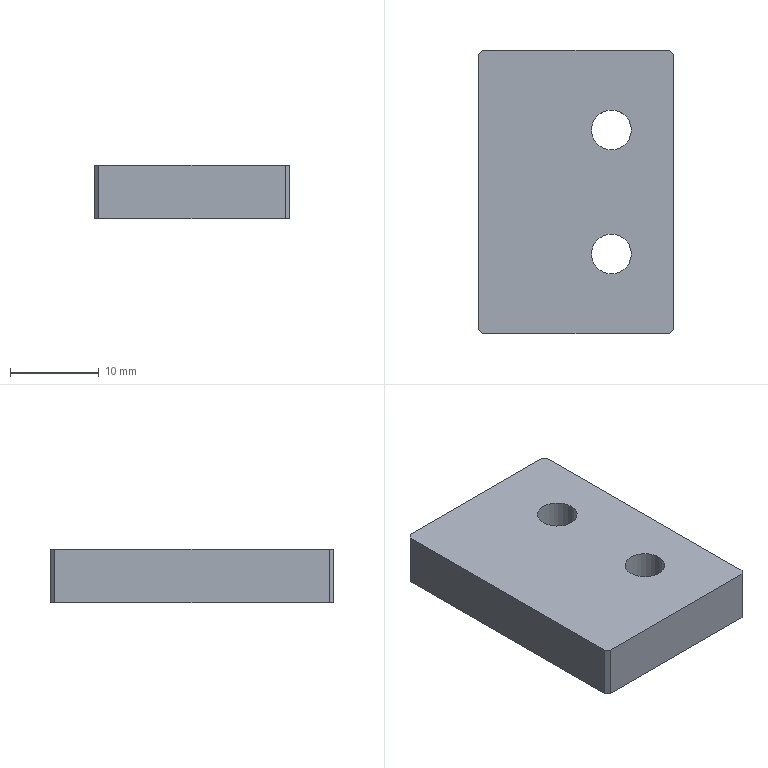Part | STEP file | PN_0014 Mount electronic clip cylinder pad block | 1 solid | 14 faces | box 22 x 32 x 6 mm | volume 4030 mm3 | plane 10 | cylinder 4 | commonest cylinder face diameters 4.5 x4
STEP:
#1=CARTESIAN_POINT('',(0.,0.,0.));
#2=DIRECTION('',(0.,0.,1.));
#3=DIRECTION('',(1.,0.,0.));
#4=AXIS2_PLACEMENT_3D('',#1,#2,#3);
#5=CARTESIAN_POINT('',(6.25,7.,0.));
#6=VERTEX_POINT('',#5);
#7=CARTESIAN_POINT('',(6.25,7.,6.));
#8=VERTEX_POINT('',#7);
#9=CARTESIAN_POINT('',(6.25,7.,6.));
#10=DIRECTION('',(0.,0.,1.));
#11=VECTOR('',#10,1.);
#12=LINE('',#9,#11);
#13=CARTESIAN_POINT('',(4.,7.,6.));
#14=DIRECTION('',(0.,0.,1.));
#15=DIRECTION('',(1.,0.,0.));
#16=AXIS2_PLACEMENT_3D('',#13,#14,#15);
#17=CYLINDRICAL_SURFACE('',#16,2.25);
#18=CARTESIAN_POINT('',(6.283,0.));
#19=DIRECTION('',(0.,1.));
#20=VECTOR('',#19,1.);
#21=LINE('',#18,#20);
#22=(GEOMETRIC_REPRESENTATION_CONTEXT(2)PARAMETRIC_REPRESENTATION_CONTEXT()REPRESENTATION_CONTEXT('',''));
#23=DEFINITIONAL_REPRESENTATION('',(#21),#22);
#24=PCURVE('',#17,#23);
#25=CARTESIAN_POINT('',(4.,7.,6.));
#26=DIRECTION('',(0.,0.,1.));
#27=DIRECTION('',(1.,0.,0.));
#28=AXIS2_PLACEMENT_3D('',#25,#26,#27);
#29=CYLINDRICAL_SURFACE('',#28,2.25);
#30=CARTESIAN_POINT('',(0.,0.));
#31=DIRECTION('',(0.,1.));
#32=VECTOR('',#31,1.);
#33=LINE('',#30,#32);
#34=(GEOMETRIC_REPRESENTATION_CONTEXT(2)PARAMETRIC_REPRESENTATION_CONTEXT()REPRESENTATION_CONTEXT('',''));
#35=DEFINITIONAL_REPRESENTATION('',(#33),#34);
#36=PCURVE('',#29,#35);
#37=SURFACE_CURVE('',#12,(#24,#36),.PCURVE_S1.);
#38=EDGE_CURVE('',#6,#8,#37,.T.);
#39=ORIENTED_EDGE('',*,*,#38,.T.);
#40=CARTESIAN_POINT('',(1.75,7.,6.));
#41=VERTEX_POINT('',#40);
#42=CARTESIAN_POINT('',(4.,7.,6.));
#43=DIRECTION('',(0.,0.,1.));
#44=DIRECTION('',(1.,0.,0.));
#45=AXIS2_PLACEMENT_3D('',#42,#43,#44);
#46=CIRCLE('',#45,2.25);
#47=CARTESIAN_POINT('',(0.,0.));
#48=DIRECTION('',(1.,0.));
#49=VECTOR('',#48,1.);
#50=LINE('',#47,#49);
#51=(GEOMETRIC_REPRESENTATION_CONTEXT(2)PARAMETRIC_REPRESENTATION_CONTEXT()REPRESENTATION_CONTEXT('',''));
#52=DEFINITIONAL_REPRESENTATION('',(#50),#51);
#53=PCURVE('',#17,#52);
#54=CARTESIAN_POINT('',(0.,0.,6.));
#55=DIRECTION('',(0.,0.,-1.));
#56=DIRECTION('',(-1.,0.,0.));
#57=AXIS2_PLACEMENT_3D('',#54,#55,#56);
#58=PLANE('',#57);
#59=CARTESIAN_POINT('',(-6.25,7.));
#60=CARTESIAN_POINT('',(-6.25,10.897));
#61=CARTESIAN_POINT('',(-2.875,8.949));
#62=CARTESIAN_POINT('',(0.5,7.));
#63=CARTESIAN_POINT('',(-2.875,5.051));
#64=CARTESIAN_POINT('',(-6.25,3.103));
#65=CARTESIAN_POINT('',(-6.25,7.));
#66=(BOUNDED_CURVE()B_SPLINE_CURVE(2,(#59,#60,#61,#62,#63,#64,#65),.UNSPECIFIED.,.T.,.F.)B_SPLINE_CURVE_WITH_KNOTS((1,2,2,2,2,1),(-2.094,0.,2.094,4.189,6.283,8.378),.UNSPECIFIED.)CURVE()GEOMETRIC_REPRESENTATION_ITEM()RATIONAL_B_SPLINE_CURVE((1.,0.5,1.,0.5,1.,0.5,1.))REPRESENTATION_ITEM(''));
#67=(GEOMETRIC_REPRESENTATION_CONTEXT(2)PARAMETRIC_REPRESENTATION_CONTEXT()REPRESENTATION_CONTEXT('',''));
#68=DEFINITIONAL_REPRESENTATION('',(#66),#67);
#69=PCURVE('',#58,#68);
#70=SURFACE_CURVE('',#46,(#53,#69),.PCURVE_S1.);
#71=EDGE_CURVE('',#41,#8,#70,.T.);
#72=ORIENTED_EDGE('',*,*,#71,.F.);
#73=CARTESIAN_POINT('',(1.75,7.,0.));
#74=VERTEX_POINT('',#73);
#75=CARTESIAN_POINT('',(1.75,7.,6.));
#76=DIRECTION('',(0.,0.,1.));
#77=VECTOR('',#76,1.);
#78=LINE('',#75,#77);
#79=CARTESIAN_POINT('',(3.142,0.));
#80=DIRECTION('',(0.,1.));
#81=VECTOR('',#80,1.);
#82=LINE('',#79,#81);
#83=(GEOMETRIC_REPRESENTATION_CONTEXT(2)PARAMETRIC_REPRESENTATION_CONTEXT()REPRESENTATION_CONTEXT('',''));
#84=DEFINITIONAL_REPRESENTATION('',(#82),#83);
#85=PCURVE('',#17,#84);
#86=CARTESIAN_POINT('',(3.142,0.));
#87=DIRECTION('',(0.,1.));
#88=VECTOR('',#87,1.);
#89=LINE('',#86,#88);
#90=(GEOMETRIC_REPRESENTATION_CONTEXT(2)PARAMETRIC_REPRESENTATION_CONTEXT()REPRESENTATION_CONTEXT('',''));
#91=DEFINITIONAL_REPRESENTATION('',(#89),#90);
#92=PCURVE('',#29,#91);
#93=SURFACE_CURVE('',#78,(#85,#92),.PCURVE_S1.);
#94=EDGE_CURVE('',#74,#41,#93,.T.);
#95=ORIENTED_EDGE('',*,*,#94,.F.);
#96=CARTESIAN_POINT('',(4.,7.,0.));
#97=DIRECTION('',(0.,0.,-1.));
#98=DIRECTION('',(-1.,0.,0.));
#99=AXIS2_PLACEMENT_3D('',#96,#97,#98);
#100=CIRCLE('',#99,2.25);
#101=CARTESIAN_POINT('',(9.425,-6.));
#102=DIRECTION('',(-1.,0.));
#103=VECTOR('',#102,1.);
#104=LINE('',#101,#103);
#105=(GEOMETRIC_REPRESENTATION_CONTEXT(2)PARAMETRIC_REPRESENTATION_CONTEXT()REPRESENTATION_CONTEXT('',''));
#106=DEFINITIONAL_REPRESENTATION('',(#104),#105);
#107=PCURVE('',#17,#106);
#108=CARTESIAN_POINT('',(0.,0.,0.));
#109=DIRECTION('',(0.,0.,-1.));
#110=DIRECTION('',(-1.,0.,0.));
#111=AXIS2_PLACEMENT_3D('',#108,#109,#110);
#112=PLANE('',#111);
#113=CARTESIAN_POINT('',(-4.,7.));
#114=DIRECTION('',(1.,0.));
#115=AXIS2_PLACEMENT_2D('',#113,#114);
#116=CIRCLE('',#115,2.25);
#117=(GEOMETRIC_REPRESENTATION_CONTEXT(2)PARAMETRIC_REPRESENTATION_CONTEXT()REPRESENTATION_CONTEXT('',''));
#118=DEFINITIONAL_REPRESENTATION('',(#116),#117);
#119=PCURVE('',#112,#118);
#120=SURFACE_CURVE('',#100,(#107,#119),.PCURVE_S1.);
#121=EDGE_CURVE('',#6,#74,#120,.T.);
#122=ORIENTED_EDGE('',*,*,#121,.F.);
#123=EDGE_LOOP('',(#39,#72,#95,#122));
#124=FACE_BOUND('',#123,.F.);
#125=ADVANCED_FACE('',(#124),#17,.F.);
#126=CARTESIAN_POINT('',(6.25,-7.,0.));
#127=VERTEX_POINT('',#126);
#128=CARTESIAN_POINT('',(6.25,-7.,6.));
#129=VERTEX_POINT('',#128);
#130=CARTESIAN_POINT('',(6.25,-7.,6.));
#131=DIRECTION('',(0.,0.,1.));
#132=VECTOR('',#131,1.);
#133=LINE('',#130,#132);
#134=CARTESIAN_POINT('',(4.,-7.,6.));
#135=DIRECTION('',(0.,0.,1.));
#136=DIRECTION('',(1.,0.,0.));
#137=AXIS2_PLACEMENT_3D('',#134,#135,#136);
#138=CYLINDRICAL_SURFACE('',#137,2.25);
#139=CARTESIAN_POINT('',(6.283,0.));
#140=DIRECTION('',(0.,1.));
#141=VECTOR('',#140,1.);
#142=LINE('',#139,#141);
#143=(GEOMETRIC_REPRESENTATION_CONTEXT(2)PARAMETRIC_REPRESENTATION_CONTEXT()REPRESENTATION_CONTEXT('',''));
#144=DEFINITIONAL_REPRESENTATION('',(#142),#143);
#145=PCURVE('',#138,#144);
#146=CARTESIAN_POINT('',(4.,-7.,6.));
#147=DIRECTION('',(0.,0.,1.));
#148=DIRECTION('',(1.,0.,0.));
#149=AXIS2_PLACEMENT_3D('',#146,#147,#148);
#150=CYLINDRICAL_SURFACE('',#149,2.25);
#151=CARTESIAN_POINT('',(0.,0.));
#152=DIRECTION('',(0.,1.));
#153=VECTOR('',#152,1.);
#154=LINE('',#151,#153);
#155=(GEOMETRIC_REPRESENTATION_CONTEXT(2)PARAMETRIC_REPRESENTATION_CONTEXT()REPRESENTATION_CONTEXT('',''));
#156=DEFINITIONAL_REPRESENTATION('',(#154),#155);
#157=PCURVE('',#150,#156);
#158=SURFACE_CURVE('',#133,(#145,#157),.PCURVE_S1.);
#159=EDGE_CURVE('',#127,#129,#158,.T.);
#160=ORIENTED_EDGE('',*,*,#159,.T.);
#161=CARTESIAN_POINT('',(1.75,-7.,6.));
#162=VERTEX_POINT('',#161);
#163=CARTESIAN_POINT('',(4.,-7.,6.));
#164=DIRECTION('',(0.,0.,1.));
#165=DIRECTION('',(1.,0.,0.));
#166=AXIS2_PLACEMENT_3D('',#163,#164,#165);
#167=CIRCLE('',#166,2.25);
#168=CARTESIAN_POINT('',(0.,0.));
#169=DIRECTION('',(1.,0.));
#170=VECTOR('',#169,1.);
#171=LINE('',#168,#170);
#172=(GEOMETRIC_REPRESENTATION_CONTEXT(2)PARAMETRIC_REPRESENTATION_CONTEXT()REPRESENTATION_CONTEXT('',''));
#173=DEFINITIONAL_REPRESENTATION('',(#171),#172);
#174=PCURVE('',#138,#173);
#175=CARTESIAN_POINT('',(-6.25,-7.));
#176=CARTESIAN_POINT('',(-6.25,-3.103));
#177=CARTESIAN_POINT('',(-2.875,-5.051));
#178=CARTESIAN_POINT('',(0.5,-7.));
#179=CARTESIAN_POINT('',(-2.875,-8.949));
#180=CARTESIAN_POINT('',(-6.25,-10.897));
#181=CARTESIAN_POINT('',(-6.25,-7.));
#182=(BOUNDED_CURVE()B_SPLINE_CURVE(2,(#175,#176,#177,#178,#179,#180,#181),.UNSPECIFIED.,.T.,.F.)B_SPLINE_CURVE_WITH_KNOTS((1,2,2,2,2,1),(-2.094,0.,2.094,4.189,6.283,8.378),.UNSPECIFIED.)CURVE()GEOMETRIC_REPRESENTATION_ITEM()RATIONAL_B_SPLINE_CURVE((1.,0.5,1.,0.5,1.,0.5,1.))REPRESENTATION_ITEM(''));
#183=(GEOMETRIC_REPRESENTATION_CONTEXT(2)PARAMETRIC_REPRESENTATION_CONTEXT()REPRESENTATION_CONTEXT('',''));
#184=DEFINITIONAL_REPRESENTATION('',(#182),#183);
#185=PCURVE('',#58,#184);
#186=SURFACE_CURVE('',#167,(#174,#185),.PCURVE_S1.);
#187=EDGE_CURVE('',#162,#129,#186,.T.);
#188=ORIENTED_EDGE('',*,*,#187,.F.);
#189=CARTESIAN_POINT('',(1.75,-7.,0.));
#190=VERTEX_POINT('',#189);
#191=CARTESIAN_POINT('',(1.75,-7.,6.));
#192=DIRECTION('',(0.,0.,1.));
#193=VECTOR('',#192,1.);
#194=LINE('',#191,#193);
#195=CARTESIAN_POINT('',(3.142,0.));
#196=DIRECTION('',(0.,1.));
#197=VECTOR('',#196,1.);
#198=LINE('',#195,#197);
#199=(GEOMETRIC_REPRESENTATION_CONTEXT(2)PARAMETRIC_REPRESENTATION_CONTEXT()REPRESENTATION_CONTEXT('',''));
#200=DEFINITIONAL_REPRESENTATION('',(#198),#199);
#201=PCURVE('',#138,#200);
#202=CARTESIAN_POINT('',(3.142,0.));
#203=DIRECTION('',(0.,1.));
#204=VECTOR('',#203,1.);
#205=LINE('',#202,#204);
#206=(GEOMETRIC_REPRESENTATION_CONTEXT(2)PARAMETRIC_REPRESENTATION_CONTEXT()REPRESENTATION_CONTEXT('',''));
#207=DEFINITIONAL_REPRESENTATION('',(#205),#206);
#208=PCURVE('',#150,#207);
#209=SURFACE_CURVE('',#194,(#201,#208),.PCURVE_S1.);
#210=EDGE_CURVE('',#190,#162,#209,.T.);
#211=ORIENTED_EDGE('',*,*,#210,.F.);
#212=CARTESIAN_POINT('',(4.,-7.,0.));
#213=DIRECTION('',(0.,0.,-1.));
#214=DIRECTION('',(-1.,0.,0.));
#215=AXIS2_PLACEMENT_3D('',#212,#213,#214);
#216=CIRCLE('',#215,2.25);
#217=CARTESIAN_POINT('',(9.425,-6.));
#218=DIRECTION('',(-1.,0.));
#219=VECTOR('',#218,1.);
#220=LINE('',#217,#219);
#221=(GEOMETRIC_REPRESENTATION_CONTEXT(2)PARAMETRIC_REPRESENTATION_CONTEXT()REPRESENTATION_CONTEXT('',''));
#222=DEFINITIONAL_REPRESENTATION('',(#220),#221);
#223=PCURVE('',#138,#222);
#224=CARTESIAN_POINT('',(-4.,-7.));
#225=DIRECTION('',(1.,0.));
#226=AXIS2_PLACEMENT_2D('',#224,#225);
#227=CIRCLE('',#226,2.25);
#228=(GEOMETRIC_REPRESENTATION_CONTEXT(2)PARAMETRIC_REPRESENTATION_CONTEXT()REPRESENTATION_CONTEXT('',''));
#229=DEFINITIONAL_REPRESENTATION('',(#227),#228);
#230=PCURVE('',#112,#229);
#231=SURFACE_CURVE('',#216,(#223,#230),.PCURVE_S1.);
#232=EDGE_CURVE('',#127,#190,#231,.T.);
#233=ORIENTED_EDGE('',*,*,#232,.F.);
#234=EDGE_LOOP('',(#160,#188,#211,#233));
#235=FACE_BOUND('',#234,.F.);
#236=ADVANCED_FACE('',(#235),#138,.F.);
#237=CARTESIAN_POINT('',(11.,-15.5,6.));
#238=VERTEX_POINT('',#237);
#239=CARTESIAN_POINT('',(11.,15.5,6.));
#240=VERTEX_POINT('',#239);
#241=CARTESIAN_POINT('',(11.,-16.,6.));
#242=DIRECTION('',(0.,1.,0.));
#243=VECTOR('',#242,1.);
#244=LINE('',#241,#243);
#245=CARTESIAN_POINT('',(11.,-16.,6.));
#246=DIRECTION('',(-1.,0.,0.));
#247=DIRECTION('',(0.,0.,1.));
#248=AXIS2_PLACEMENT_3D('',#245,#246,#247);
#249=PLANE('',#248);
#250=CARTESIAN_POINT('',(0.,0.));
#251=DIRECTION('',(0.,1.));
#252=VECTOR('',#251,1.);
#253=LINE('',#250,#252);
#254=(GEOMETRIC_REPRESENTATION_CONTEXT(2)PARAMETRIC_REPRESENTATION_CONTEXT()REPRESENTATION_CONTEXT('',''));
#255=DEFINITIONAL_REPRESENTATION('',(#253),#254);
#256=PCURVE('',#249,#255);
#257=CARTESIAN_POINT('',(-11.,-16.));
#258=DIRECTION('',(0.,1.));
#259=VECTOR('',#258,1.);
#260=LINE('',#257,#259);
#261=(GEOMETRIC_REPRESENTATION_CONTEXT(2)PARAMETRIC_REPRESENTATION_CONTEXT()REPRESENTATION_CONTEXT('',''));
#262=DEFINITIONAL_REPRESENTATION('',(#260),#261);
#263=PCURVE('',#58,#262);
#264=SURFACE_CURVE('',#244,(#256,#263),.PCURVE_S1.);
#265=EDGE_CURVE('',#238,#240,#264,.T.);
#266=ORIENTED_EDGE('',*,*,#265,.F.);
#267=CARTESIAN_POINT('',(11.,-15.5,0.));
#268=VERTEX_POINT('',#267);
#269=CARTESIAN_POINT('',(11.,-15.5,6.));
#270=DIRECTION('',(0.,0.,-1.));
#271=VECTOR('',#270,1.);
#272=LINE('',#269,#271);
#273=CARTESIAN_POINT('',(0.,0.5));
#274=DIRECTION('',(-1.,0.));
#275=VECTOR('',#274,1.);
#276=LINE('',#273,#275);
#277=(GEOMETRIC_REPRESENTATION_CONTEXT(2)PARAMETRIC_REPRESENTATION_CONTEXT()REPRESENTATION_CONTEXT('',''));
#278=DEFINITIONAL_REPRESENTATION('',(#276),#277);
#279=PCURVE('',#249,#278);
#280=CARTESIAN_POINT('',(11.,-15.5,6.));
#281=DIRECTION('',(-0.7071,0.7071,0.));
#282=DIRECTION('',(0.,0.,-1.));
#283=AXIS2_PLACEMENT_3D('',#280,#281,#282);
#284=PLANE('',#283);
#285=CARTESIAN_POINT('',(0.,0.));
#286=DIRECTION('',(1.,0.));
#287=VECTOR('',#286,1.);
#288=LINE('',#285,#287);
#289=(GEOMETRIC_REPRESENTATION_CONTEXT(2)PARAMETRIC_REPRESENTATION_CONTEXT()REPRESENTATION_CONTEXT('',''));
#290=DEFINITIONAL_REPRESENTATION('',(#288),#289);
#291=PCURVE('',#284,#290);
#292=SURFACE_CURVE('',#272,(#279,#291),.PCURVE_S1.);
#293=EDGE_CURVE('',#238,#268,#292,.T.);
#294=ORIENTED_EDGE('',*,*,#293,.T.);
#295=CARTESIAN_POINT('',(11.,15.5,0.));
#296=VERTEX_POINT('',#295);
#297=CARTESIAN_POINT('',(11.,-16.,0.));
#298=DIRECTION('',(0.,1.,0.));
#299=VECTOR('',#298,1.);
#300=LINE('',#297,#299);
#301=CARTESIAN_POINT('',(-6.,0.));
#302=DIRECTION('',(0.,1.));
#303=VECTOR('',#302,1.);
#304=LINE('',#301,#303);
#305=(GEOMETRIC_REPRESENTATION_CONTEXT(2)PARAMETRIC_REPRESENTATION_CONTEXT()REPRESENTATION_CONTEXT('',''));
#306=DEFINITIONAL_REPRESENTATION('',(#304),#305);
#307=PCURVE('',#249,#306);
#308=CARTESIAN_POINT('',(-11.,-16.));
#309=DIRECTION('',(0.,1.));
#310=VECTOR('',#309,1.);
#311=LINE('',#308,#310);
#312=(GEOMETRIC_REPRESENTATION_CONTEXT(2)PARAMETRIC_REPRESENTATION_CONTEXT()REPRESENTATION_CONTEXT('',''));
#313=DEFINITIONAL_REPRESENTATION('',(#311),#312);
#314=PCURVE('',#112,#313);
#315=SURFACE_CURVE('',#300,(#307,#314),.PCURVE_S1.);
#316=EDGE_CURVE('',#268,#296,#315,.T.);
#317=ORIENTED_EDGE('',*,*,#316,.T.);
#318=CARTESIAN_POINT('',(11.,15.5,6.));
#319=DIRECTION('',(0.,0.,1.));
#320=VECTOR('',#319,1.);
#321=LINE('',#318,#320);
#322=CARTESIAN_POINT('',(0.,31.5));
#323=DIRECTION('',(1.,0.));
#324=VECTOR('',#323,1.);
#325=LINE('',#322,#324);
#326=(GEOMETRIC_REPRESENTATION_CONTEXT(2)PARAMETRIC_REPRESENTATION_CONTEXT()REPRESENTATION_CONTEXT('',''));
#327=DEFINITIONAL_REPRESENTATION('',(#325),#326);
#328=PCURVE('',#249,#327);
#329=CARTESIAN_POINT('',(10.5,16.,6.));
#330=DIRECTION('',(-0.7071,-0.7071,0.));
#331=DIRECTION('',(0.,0.,-1.));
#332=AXIS2_PLACEMENT_3D('',#329,#330,#331);
#333=PLANE('',#332);
#334=CARTESIAN_POINT('',(0.,0.7071));
#335=DIRECTION('',(-1.,0.));
#336=VECTOR('',#335,1.);
#337=LINE('',#334,#336);
#338=(GEOMETRIC_REPRESENTATION_CONTEXT(2)PARAMETRIC_REPRESENTATION_CONTEXT()REPRESENTATION_CONTEXT('',''));
#339=DEFINITIONAL_REPRESENTATION('',(#337),#338);
#340=PCURVE('',#333,#339);
#341=SURFACE_CURVE('',#321,(#328,#340),.PCURVE_S1.);
#342=EDGE_CURVE('',#296,#240,#341,.T.);
#343=ORIENTED_EDGE('',*,*,#342,.T.);
#344=EDGE_LOOP('',(#266,#294,#317,#343));
#345=FACE_BOUND('',#344,.T.);
#346=ADVANCED_FACE('',(#345),#249,.F.);
#347=CARTESIAN_POINT('',(10.5,16.,0.));
#348=VERTEX_POINT('',#347);
#349=CARTESIAN_POINT('',(-10.5,16.,0.));
#350=VERTEX_POINT('',#349);
#351=CARTESIAN_POINT('',(-11.,16.,0.));
#352=DIRECTION('',(-1.,0.,0.));
#353=VECTOR('',#352,1.);
#354=LINE('',#351,#353);
#355=CARTESIAN_POINT('',(-11.,16.,6.));
#356=DIRECTION('',(0.,-1.,0.));
#357=DIRECTION('',(0.,0.,-1.));
#358=AXIS2_PLACEMENT_3D('',#355,#356,#357);
#359=PLANE('',#358);
#360=CARTESIAN_POINT('',(6.,0.));
#361=DIRECTION('',(0.,-1.));
#362=VECTOR('',#361,1.);
#363=LINE('',#360,#362);
#364=(GEOMETRIC_REPRESENTATION_CONTEXT(2)PARAMETRIC_REPRESENTATION_CONTEXT()REPRESENTATION_CONTEXT('',''));
#365=DEFINITIONAL_REPRESENTATION('',(#363),#364);
#366=PCURVE('',#359,#365);
#367=CARTESIAN_POINT('',(11.,16.));
#368=DIRECTION('',(1.,0.));
#369=VECTOR('',#368,1.);
#370=LINE('',#367,#369);
#371=(GEOMETRIC_REPRESENTATION_CONTEXT(2)PARAMETRIC_REPRESENTATION_CONTEXT()REPRESENTATION_CONTEXT('',''));
#372=DEFINITIONAL_REPRESENTATION('',(#370),#371);
#373=PCURVE('',#112,#372);
#374=SURFACE_CURVE('',#354,(#366,#373),.PCURVE_S1.);
#375=EDGE_CURVE('',#348,#350,#374,.T.);
#376=ORIENTED_EDGE('',*,*,#375,.T.);
#377=CARTESIAN_POINT('',(-10.5,16.,6.));
#378=VERTEX_POINT('',#377);
#379=CARTESIAN_POINT('',(-10.5,16.,6.));
#380=DIRECTION('',(0.,0.,1.));
#381=VECTOR('',#380,1.);
#382=LINE('',#379,#381);
#383=CARTESIAN_POINT('',(0.,0.5));
#384=DIRECTION('',(-1.,0.));
#385=VECTOR('',#384,1.);
#386=LINE('',#383,#385);
#387=(GEOMETRIC_REPRESENTATION_CONTEXT(2)PARAMETRIC_REPRESENTATION_CONTEXT()REPRESENTATION_CONTEXT('',''));
#388=DEFINITIONAL_REPRESENTATION('',(#386),#387);
#389=PCURVE('',#359,#388);
#390=CARTESIAN_POINT('',(-11.,15.5,6.));
#391=DIRECTION('',(0.7071,-0.7071,0.));
#392=DIRECTION('',(0.,0.,-1.));
#393=AXIS2_PLACEMENT_3D('',#390,#391,#392);
#394=PLANE('',#393);
#395=CARTESIAN_POINT('',(0.,0.7071));
#396=DIRECTION('',(-1.,0.));
#397=VECTOR('',#396,1.);
#398=LINE('',#395,#397);
#399=(GEOMETRIC_REPRESENTATION_CONTEXT(2)PARAMETRIC_REPRESENTATION_CONTEXT()REPRESENTATION_CONTEXT('',''));
#400=DEFINITIONAL_REPRESENTATION('',(#398),#399);
#401=PCURVE('',#394,#400);
#402=SURFACE_CURVE('',#382,(#389,#401),.PCURVE_S1.);
#403=EDGE_CURVE('',#350,#378,#402,.T.);
#404=ORIENTED_EDGE('',*,*,#403,.T.);
#405=CARTESIAN_POINT('',(10.5,16.,6.));
#406=VERTEX_POINT('',#405);
#407=CARTESIAN_POINT('',(-11.,16.,6.));
#408=DIRECTION('',(-1.,0.,0.));
#409=VECTOR('',#408,1.);
#410=LINE('',#407,#409);
#411=CARTESIAN_POINT('',(0.,0.));
#412=DIRECTION('',(0.,-1.));
#413=VECTOR('',#412,1.);
#414=LINE('',#411,#413);
#415=(GEOMETRIC_REPRESENTATION_CONTEXT(2)PARAMETRIC_REPRESENTATION_CONTEXT()REPRESENTATION_CONTEXT('',''));
#416=DEFINITIONAL_REPRESENTATION('',(#414),#415);
#417=PCURVE('',#359,#416);
#418=CARTESIAN_POINT('',(11.,16.));
#419=DIRECTION('',(1.,0.));
#420=VECTOR('',#419,1.);
#421=LINE('',#418,#420);
#422=(GEOMETRIC_REPRESENTATION_CONTEXT(2)PARAMETRIC_REPRESENTATION_CONTEXT()REPRESENTATION_CONTEXT('',''));
#423=DEFINITIONAL_REPRESENTATION('',(#421),#422);
#424=PCURVE('',#58,#423);
#425=SURFACE_CURVE('',#410,(#417,#424),.PCURVE_S1.);
#426=EDGE_CURVE('',#406,#378,#425,.T.);
#427=ORIENTED_EDGE('',*,*,#426,.F.);
#428=CARTESIAN_POINT('',(10.5,16.,6.));
#429=DIRECTION('',(0.,0.,-1.));
#430=VECTOR('',#429,1.);
#431=LINE('',#428,#430);
#432=CARTESIAN_POINT('',(0.,21.5));
#433=DIRECTION('',(1.,0.));
#434=VECTOR('',#433,1.);
#435=LINE('',#432,#434);
#436=(GEOMETRIC_REPRESENTATION_CONTEXT(2)PARAMETRIC_REPRESENTATION_CONTEXT()REPRESENTATION_CONTEXT('',''));
#437=DEFINITIONAL_REPRESENTATION('',(#435),#436);
#438=PCURVE('',#359,#437);
#439=CARTESIAN_POINT('',(0.,0.));
#440=DIRECTION('',(1.,0.));
#441=VECTOR('',#440,1.);
#442=LINE('',#439,#441);
#443=(GEOMETRIC_REPRESENTATION_CONTEXT(2)PARAMETRIC_REPRESENTATION_CONTEXT()REPRESENTATION_CONTEXT('',''));
#444=DEFINITIONAL_REPRESENTATION('',(#442),#443);
#445=PCURVE('',#333,#444);
#446=SURFACE_CURVE('',#431,(#438,#445),.PCURVE_S1.);
#447=EDGE_CURVE('',#406,#348,#446,.T.);
#448=ORIENTED_EDGE('',*,*,#447,.T.);
#449=EDGE_LOOP('',(#376,#404,#427,#448));
#450=FACE_BOUND('',#449,.T.);
#451=ADVANCED_FACE('',(#450),#359,.F.);
#452=CARTESIAN_POINT('',(-11.,15.5,0.));
#453=VERTEX_POINT('',#452);
#454=CARTESIAN_POINT('',(-11.,-15.5,0.));
#455=VERTEX_POINT('',#454);
#456=CARTESIAN_POINT('',(-11.,-16.,0.));
#457=DIRECTION('',(0.,-1.,0.));
#458=VECTOR('',#457,1.);
#459=LINE('',#456,#458);
#460=CARTESIAN_POINT('',(-11.,-16.,6.));
#461=DIRECTION('',(1.,0.,0.));
#462=DIRECTION('',(0.,0.,-1.));
#463=AXIS2_PLACEMENT_3D('',#460,#461,#462);
#464=PLANE('',#463);
#465=CARTESIAN_POINT('',(6.,0.));
#466=DIRECTION('',(0.,-1.));
#467=VECTOR('',#466,1.);
#468=LINE('',#465,#467);
#469=(GEOMETRIC_REPRESENTATION_CONTEXT(2)PARAMETRIC_REPRESENTATION_CONTEXT()REPRESENTATION_CONTEXT('',''));
#470=DEFINITIONAL_REPRESENTATION('',(#468),#469);
#471=PCURVE('',#464,#470);
#472=CARTESIAN_POINT('',(11.,-16.));
#473=DIRECTION('',(0.,-1.));
#474=VECTOR('',#473,1.);
#475=LINE('',#472,#474);
#476=(GEOMETRIC_REPRESENTATION_CONTEXT(2)PARAMETRIC_REPRESENTATION_CONTEXT()REPRESENTATION_CONTEXT('',''));
#477=DEFINITIONAL_REPRESENTATION('',(#475),#476);
#478=PCURVE('',#112,#477);
#479=SURFACE_CURVE('',#459,(#471,#478),.PCURVE_S1.);
#480=EDGE_CURVE('',#453,#455,#479,.T.);
#481=ORIENTED_EDGE('',*,*,#480,.T.);
#482=CARTESIAN_POINT('',(-11.,-15.5,6.));
#483=VERTEX_POINT('',#482);
#484=CARTESIAN_POINT('',(-11.,-15.5,6.));
#485=DIRECTION('',(0.,0.,1.));
#486=VECTOR('',#485,1.);
#487=LINE('',#484,#486);
#488=CARTESIAN_POINT('',(0.,0.5));
#489=DIRECTION('',(-1.,0.));
#490=VECTOR('',#489,1.);
#491=LINE('',#488,#490);
#492=(GEOMETRIC_REPRESENTATION_CONTEXT(2)PARAMETRIC_REPRESENTATION_CONTEXT()REPRESENTATION_CONTEXT('',''));
#493=DEFINITIONAL_REPRESENTATION('',(#491),#492);
#494=PCURVE('',#464,#493);
#495=CARTESIAN_POINT('',(-10.5,-16.,6.));
#496=DIRECTION('',(0.7071,0.7071,0.));
#497=DIRECTION('',(0.,0.,-1.));
#498=AXIS2_PLACEMENT_3D('',#495,#496,#497);
#499=PLANE('',#498);
#500=CARTESIAN_POINT('',(0.,0.7071));
#501=DIRECTION('',(-1.,0.));
#502=VECTOR('',#501,1.);
#503=LINE('',#500,#502);
#504=(GEOMETRIC_REPRESENTATION_CONTEXT(2)PARAMETRIC_REPRESENTATION_CONTEXT()REPRESENTATION_CONTEXT('',''));
#505=DEFINITIONAL_REPRESENTATION('',(#503),#504);
#506=PCURVE('',#499,#505);
#507=SURFACE_CURVE('',#487,(#494,#506),.PCURVE_S1.);
#508=EDGE_CURVE('',#455,#483,#507,.T.);
#509=ORIENTED_EDGE('',*,*,#508,.T.);
#510=CARTESIAN_POINT('',(-11.,15.5,6.));
#511=VERTEX_POINT('',#510);
#512=CARTESIAN_POINT('',(-11.,-16.,6.));
#513=DIRECTION('',(0.,-1.,0.));
#514=VECTOR('',#513,1.);
#515=LINE('',#512,#514);
#516=CARTESIAN_POINT('',(0.,0.));
#517=DIRECTION('',(0.,-1.));
#518=VECTOR('',#517,1.);
#519=LINE('',#516,#518);
#520=(GEOMETRIC_REPRESENTATION_CONTEXT(2)PARAMETRIC_REPRESENTATION_CONTEXT()REPRESENTATION_CONTEXT('',''));
#521=DEFINITIONAL_REPRESENTATION('',(#519),#520);
#522=PCURVE('',#464,#521);
#523=CARTESIAN_POINT('',(11.,-16.));
#524=DIRECTION('',(0.,-1.));
#525=VECTOR('',#524,1.);
#526=LINE('',#523,#525);
#527=(GEOMETRIC_REPRESENTATION_CONTEXT(2)PARAMETRIC_REPRESENTATION_CONTEXT()REPRESENTATION_CONTEXT('',''));
#528=DEFINITIONAL_REPRESENTATION('',(#526),#527);
#529=PCURVE('',#58,#528);
#530=SURFACE_CURVE('',#515,(#522,#529),.PCURVE_S1.);
#531=EDGE_CURVE('',#511,#483,#530,.T.);
#532=ORIENTED_EDGE('',*,*,#531,.F.);
#533=CARTESIAN_POINT('',(-11.,15.5,6.));
#534=DIRECTION('',(0.,0.,-1.));
#535=VECTOR('',#534,1.);
#536=LINE('',#533,#535);
#537=CARTESIAN_POINT('',(0.,31.5));
#538=DIRECTION('',(1.,0.));
#539=VECTOR('',#538,1.);
#540=LINE('',#537,#539);
#541=(GEOMETRIC_REPRESENTATION_CONTEXT(2)PARAMETRIC_REPRESENTATION_CONTEXT()REPRESENTATION_CONTEXT('',''));
#542=DEFINITIONAL_REPRESENTATION('',(#540),#541);
#543=PCURVE('',#464,#542);
#544=CARTESIAN_POINT('',(0.,0.));
#545=DIRECTION('',(1.,0.));
#546=VECTOR('',#545,1.);
#547=LINE('',#544,#546);
#548=(GEOMETRIC_REPRESENTATION_CONTEXT(2)PARAMETRIC_REPRESENTATION_CONTEXT()REPRESENTATION_CONTEXT('',''));
#549=DEFINITIONAL_REPRESENTATION('',(#547),#548);
#550=PCURVE('',#394,#549);
#551=SURFACE_CURVE('',#536,(#543,#550),.PCURVE_S1.);
#552=EDGE_CURVE('',#511,#453,#551,.T.);
#553=ORIENTED_EDGE('',*,*,#552,.T.);
#554=EDGE_LOOP('',(#481,#509,#532,#553));
#555=FACE_BOUND('',#554,.T.);
#556=ADVANCED_FACE('',(#555),#464,.F.);
#557=CARTESIAN_POINT('',(-10.5,-16.,0.));
#558=VERTEX_POINT('',#557);
#559=CARTESIAN_POINT('',(10.5,-16.,0.));
#560=VERTEX_POINT('',#559);
#561=CARTESIAN_POINT('',(-11.,-16.,0.));
#562=DIRECTION('',(1.,0.,0.));
#563=VECTOR('',#562,1.);
#564=LINE('',#561,#563);
#565=CARTESIAN_POINT('',(-11.,-16.,6.));
#566=DIRECTION('',(0.,1.,0.));
#567=DIRECTION('',(0.,0.,1.));
#568=AXIS2_PLACEMENT_3D('',#565,#566,#567);
#569=PLANE('',#568);
#570=CARTESIAN_POINT('',(-6.,0.));
#571=DIRECTION('',(0.,1.));
#572=VECTOR('',#571,1.);
#573=LINE('',#570,#572);
#574=(GEOMETRIC_REPRESENTATION_CONTEXT(2)PARAMETRIC_REPRESENTATION_CONTEXT()REPRESENTATION_CONTEXT('',''));
#575=DEFINITIONAL_REPRESENTATION('',(#573),#574);
#576=PCURVE('',#569,#575);
#577=CARTESIAN_POINT('',(11.,-16.));
#578=DIRECTION('',(-1.,0.));
#579=VECTOR('',#578,1.);
#580=LINE('',#577,#579);
#581=(GEOMETRIC_REPRESENTATION_CONTEXT(2)PARAMETRIC_REPRESENTATION_CONTEXT()REPRESENTATION_CONTEXT('',''));
#582=DEFINITIONAL_REPRESENTATION('',(#580),#581);
#583=PCURVE('',#112,#582);
#584=SURFACE_CURVE('',#564,(#576,#583),.PCURVE_S1.);
#585=EDGE_CURVE('',#558,#560,#584,.T.);
#586=ORIENTED_EDGE('',*,*,#585,.T.);
#587=CARTESIAN_POINT('',(10.5,-16.,6.));
#588=VERTEX_POINT('',#587);
#589=CARTESIAN_POINT('',(10.5,-16.,6.));
#590=DIRECTION('',(0.,0.,1.));
#591=VECTOR('',#590,1.);
#592=LINE('',#589,#591);
#593=CARTESIAN_POINT('',(0.,21.5));
#594=DIRECTION('',(1.,0.));
#595=VECTOR('',#594,1.);
#596=LINE('',#593,#595);
#597=(GEOMETRIC_REPRESENTATION_CONTEXT(2)PARAMETRIC_REPRESENTATION_CONTEXT()REPRESENTATION_CONTEXT('',''));
#598=DEFINITIONAL_REPRESENTATION('',(#596),#597);
#599=PCURVE('',#569,#598);
#600=CARTESIAN_POINT('',(0.,0.7071));
#601=DIRECTION('',(-1.,0.));
#602=VECTOR('',#601,1.);
#603=LINE('',#600,#602);
#604=(GEOMETRIC_REPRESENTATION_CONTEXT(2)PARAMETRIC_REPRESENTATION_CONTEXT()REPRESENTATION_CONTEXT('',''));
#605=DEFINITIONAL_REPRESENTATION('',(#603),#604);
#606=PCURVE('',#284,#605);
#607=SURFACE_CURVE('',#592,(#599,#606),.PCURVE_S1.);
#608=EDGE_CURVE('',#560,#588,#607,.T.);
#609=ORIENTED_EDGE('',*,*,#608,.T.);
#610=CARTESIAN_POINT('',(-10.5,-16.,6.));
#611=VERTEX_POINT('',#610);
#612=CARTESIAN_POINT('',(-11.,-16.,6.));
#613=DIRECTION('',(1.,0.,0.));
#614=VECTOR('',#613,1.);
#615=LINE('',#612,#614);
#616=CARTESIAN_POINT('',(0.,0.));
#617=DIRECTION('',(0.,1.));
#618=VECTOR('',#617,1.);
#619=LINE('',#616,#618);
#620=(GEOMETRIC_REPRESENTATION_CONTEXT(2)PARAMETRIC_REPRESENTATION_CONTEXT()REPRESENTATION_CONTEXT('',''));
#621=DEFINITIONAL_REPRESENTATION('',(#619),#620);
#622=PCURVE('',#569,#621);
#623=CARTESIAN_POINT('',(11.,-16.));
#624=DIRECTION('',(-1.,0.));
#625=VECTOR('',#624,1.);
#626=LINE('',#623,#625);
#627=(GEOMETRIC_REPRESENTATION_CONTEXT(2)PARAMETRIC_REPRESENTATION_CONTEXT()REPRESENTATION_CONTEXT('',''));
#628=DEFINITIONAL_REPRESENTATION('',(#626),#627);
#629=PCURVE('',#58,#628);
#630=SURFACE_CURVE('',#615,(#622,#629),.PCURVE_S1.);
#631=EDGE_CURVE('',#611,#588,#630,.T.);
#632=ORIENTED_EDGE('',*,*,#631,.F.);
#633=CARTESIAN_POINT('',(-10.5,-16.,6.));
#634=DIRECTION('',(0.,0.,-1.));
#635=VECTOR('',#634,1.);
#636=LINE('',#633,#635);
#637=CARTESIAN_POINT('',(0.,0.5));
#638=DIRECTION('',(-1.,0.));
#639=VECTOR('',#638,1.);
#640=LINE('',#637,#639);
#641=(GEOMETRIC_REPRESENTATION_CONTEXT(2)PARAMETRIC_REPRESENTATION_CONTEXT()REPRESENTATION_CONTEXT('',''));
#642=DEFINITIONAL_REPRESENTATION('',(#640),#641);
#643=PCURVE('',#569,#642);
#644=CARTESIAN_POINT('',(0.,0.));
#645=DIRECTION('',(1.,0.));
#646=VECTOR('',#645,1.);
#647=LINE('',#644,#646);
#648=(GEOMETRIC_REPRESENTATION_CONTEXT(2)PARAMETRIC_REPRESENTATION_CONTEXT()REPRESENTATION_CONTEXT('',''));
#649=DEFINITIONAL_REPRESENTATION('',(#647),#648);
#650=PCURVE('',#499,#649);
#651=SURFACE_CURVE('',#636,(#643,#650),.PCURVE_S1.);
#652=EDGE_CURVE('',#611,#558,#651,.T.);
#653=ORIENTED_EDGE('',*,*,#652,.T.);
#654=EDGE_LOOP('',(#586,#609,#632,#653));
#655=FACE_BOUND('',#654,.T.);
#656=ADVANCED_FACE('',(#655),#569,.F.);
#657=CARTESIAN_POINT('',(4.,7.,6.));
#658=DIRECTION('',(0.,0.,1.));
#659=DIRECTION('',(1.,0.,0.));
#660=AXIS2_PLACEMENT_3D('',#657,#658,#659);
#661=CIRCLE('',#660,2.25);
#662=CARTESIAN_POINT('',(-6.25,7.));
#663=CARTESIAN_POINT('',(-6.25,10.897));
#664=CARTESIAN_POINT('',(-2.875,8.949));
#665=CARTESIAN_POINT('',(0.5,7.));
#666=CARTESIAN_POINT('',(-2.875,5.051));
#667=CARTESIAN_POINT('',(-6.25,3.103));
#668=CARTESIAN_POINT('',(-6.25,7.));
#669=(BOUNDED_CURVE()B_SPLINE_CURVE(2,(#662,#663,#664,#665,#666,#667,#668),.UNSPECIFIED.,.T.,.F.)B_SPLINE_CURVE_WITH_KNOTS((1,2,2,2,2,1),(-2.094,0.,2.094,4.189,6.283,8.378),.UNSPECIFIED.)CURVE()GEOMETRIC_REPRESENTATION_ITEM()RATIONAL_B_SPLINE_CURVE((1.,0.5,1.,0.5,1.,0.5,1.))REPRESENTATION_ITEM(''));
#670=(GEOMETRIC_REPRESENTATION_CONTEXT(2)PARAMETRIC_REPRESENTATION_CONTEXT()REPRESENTATION_CONTEXT('',''));
#671=DEFINITIONAL_REPRESENTATION('',(#669),#670);
#672=PCURVE('',#58,#671);
#673=CARTESIAN_POINT('',(0.,0.));
#674=DIRECTION('',(1.,0.));
#675=VECTOR('',#674,1.);
#676=LINE('',#673,#675);
#677=(GEOMETRIC_REPRESENTATION_CONTEXT(2)PARAMETRIC_REPRESENTATION_CONTEXT()REPRESENTATION_CONTEXT('',''));
#678=DEFINITIONAL_REPRESENTATION('',(#676),#677);
#679=PCURVE('',#29,#678);
#680=SURFACE_CURVE('',#661,(#672,#679),.PCURVE_S1.);
#681=EDGE_CURVE('',#8,#41,#680,.T.);
#682=ORIENTED_EDGE('',*,*,#681,.F.);
#683=ORIENTED_EDGE('',*,*,#71,.F.);
#684=EDGE_LOOP('',(#682,#683));
#685=FACE_BOUND('',#684,.T.);
#686=CARTESIAN_POINT('',(4.,-7.,6.));
#687=DIRECTION('',(0.,0.,1.));
#688=DIRECTION('',(1.,0.,0.));
#689=AXIS2_PLACEMENT_3D('',#686,#687,#688);
#690=CIRCLE('',#689,2.25);
#691=CARTESIAN_POINT('',(-6.25,-7.));
#692=CARTESIAN_POINT('',(-6.25,-3.103));
#693=CARTESIAN_POINT('',(-2.875,-5.051));
#694=CARTESIAN_POINT('',(0.5,-7.));
#695=CARTESIAN_POINT('',(-2.875,-8.949));
#696=CARTESIAN_POINT('',(-6.25,-10.897));
#697=CARTESIAN_POINT('',(-6.25,-7.));
#698=(BOUNDED_CURVE()B_SPLINE_CURVE(2,(#691,#692,#693,#694,#695,#696,#697),.UNSPECIFIED.,.T.,.F.)B_SPLINE_CURVE_WITH_KNOTS((1,2,2,2,2,1),(-2.094,0.,2.094,4.189,6.283,8.378),.UNSPECIFIED.)CURVE()GEOMETRIC_REPRESENTATION_ITEM()RATIONAL_B_SPLINE_CURVE((1.,0.5,1.,0.5,1.,0.5,1.))REPRESENTATION_ITEM(''));
#699=(GEOMETRIC_REPRESENTATION_CONTEXT(2)PARAMETRIC_REPRESENTATION_CONTEXT()REPRESENTATION_CONTEXT('',''));
#700=DEFINITIONAL_REPRESENTATION('',(#698),#699);
#701=PCURVE('',#58,#700);
#702=CARTESIAN_POINT('',(0.,0.));
#703=DIRECTION('',(1.,0.));
#704=VECTOR('',#703,1.);
#705=LINE('',#702,#704);
#706=(GEOMETRIC_REPRESENTATION_CONTEXT(2)PARAMETRIC_REPRESENTATION_CONTEXT()REPRESENTATION_CONTEXT('',''));
#707=DEFINITIONAL_REPRESENTATION('',(#705),#706);
#708=PCURVE('',#150,#707);
#709=SURFACE_CURVE('',#690,(#701,#708),.PCURVE_S1.);
#710=EDGE_CURVE('',#129,#162,#709,.T.);
#711=ORIENTED_EDGE('',*,*,#710,.F.);
#712=ORIENTED_EDGE('',*,*,#187,.F.);
#713=EDGE_LOOP('',(#711,#712));
#714=FACE_BOUND('',#713,.T.);
#715=ORIENTED_EDGE('',*,*,#631,.T.);
#716=CARTESIAN_POINT('',(11.,-15.5,6.));
#717=DIRECTION('',(0.7071,0.7071,0.));
#718=VECTOR('',#717,1.);
#719=LINE('',#716,#718);
#720=CARTESIAN_POINT('',(-11.,-15.5));
#721=DIRECTION('',(-0.7071,0.7071));
#722=VECTOR('',#721,1.);
#723=LINE('',#720,#722);
#724=(GEOMETRIC_REPRESENTATION_CONTEXT(2)PARAMETRIC_REPRESENTATION_CONTEXT()REPRESENTATION_CONTEXT('',''));
#725=DEFINITIONAL_REPRESENTATION('',(#723),#724);
#726=PCURVE('',#58,#725);
#727=CARTESIAN_POINT('',(0.,0.));
#728=DIRECTION('',(0.,-1.));
#729=VECTOR('',#728,1.);
#730=LINE('',#727,#729);
#731=(GEOMETRIC_REPRESENTATION_CONTEXT(2)PARAMETRIC_REPRESENTATION_CONTEXT()REPRESENTATION_CONTEXT('',''));
#732=DEFINITIONAL_REPRESENTATION('',(#730),#731);
#733=PCURVE('',#284,#732);
#734=SURFACE_CURVE('',#719,(#726,#733),.PCURVE_S1.);
#735=EDGE_CURVE('',#588,#238,#734,.T.);
#736=ORIENTED_EDGE('',*,*,#735,.T.);
#737=ORIENTED_EDGE('',*,*,#265,.T.);
#738=CARTESIAN_POINT('',(10.5,16.,6.));
#739=DIRECTION('',(-0.7071,0.7071,0.));
#740=VECTOR('',#739,1.);
#741=LINE('',#738,#740);
#742=CARTESIAN_POINT('',(-10.5,16.));
#743=DIRECTION('',(0.7071,0.7071));
#744=VECTOR('',#743,1.);
#745=LINE('',#742,#744);
#746=(GEOMETRIC_REPRESENTATION_CONTEXT(2)PARAMETRIC_REPRESENTATION_CONTEXT()REPRESENTATION_CONTEXT('',''));
#747=DEFINITIONAL_REPRESENTATION('',(#745),#746);
#748=PCURVE('',#58,#747);
#749=CARTESIAN_POINT('',(0.,0.));
#750=DIRECTION('',(0.,-1.));
#751=VECTOR('',#750,1.);
#752=LINE('',#749,#751);
#753=(GEOMETRIC_REPRESENTATION_CONTEXT(2)PARAMETRIC_REPRESENTATION_CONTEXT()REPRESENTATION_CONTEXT('',''));
#754=DEFINITIONAL_REPRESENTATION('',(#752),#753);
#755=PCURVE('',#333,#754);
#756=SURFACE_CURVE('',#741,(#748,#755),.PCURVE_S1.);
#757=EDGE_CURVE('',#240,#406,#756,.T.);
#758=ORIENTED_EDGE('',*,*,#757,.T.);
#759=ORIENTED_EDGE('',*,*,#426,.T.);
#760=CARTESIAN_POINT('',(-11.,15.5,6.));
#761=DIRECTION('',(-0.7071,-0.7071,0.));
#762=VECTOR('',#761,1.);
#763=LINE('',#760,#762);
#764=CARTESIAN_POINT('',(11.,15.5));
#765=DIRECTION('',(0.7071,-0.7071));
#766=VECTOR('',#765,1.);
#767=LINE('',#764,#766);
#768=(GEOMETRIC_REPRESENTATION_CONTEXT(2)PARAMETRIC_REPRESENTATION_CONTEXT()REPRESENTATION_CONTEXT('',''));
#769=DEFINITIONAL_REPRESENTATION('',(#767),#768);
#770=PCURVE('',#58,#769);
#771=CARTESIAN_POINT('',(0.,0.));
#772=DIRECTION('',(0.,-1.));
#773=VECTOR('',#772,1.);
#774=LINE('',#771,#773);
#775=(GEOMETRIC_REPRESENTATION_CONTEXT(2)PARAMETRIC_REPRESENTATION_CONTEXT()REPRESENTATION_CONTEXT('',''));
#776=DEFINITIONAL_REPRESENTATION('',(#774),#775);
#777=PCURVE('',#394,#776);
#778=SURFACE_CURVE('',#763,(#770,#777),.PCURVE_S1.);
#779=EDGE_CURVE('',#378,#511,#778,.T.);
#780=ORIENTED_EDGE('',*,*,#779,.T.);
#781=ORIENTED_EDGE('',*,*,#531,.T.);
#782=CARTESIAN_POINT('',(-10.5,-16.,6.));
#783=DIRECTION('',(0.7071,-0.7071,0.));
#784=VECTOR('',#783,1.);
#785=LINE('',#782,#784);
#786=CARTESIAN_POINT('',(10.5,-16.));
#787=DIRECTION('',(-0.7071,-0.7071));
#788=VECTOR('',#787,1.);
#789=LINE('',#786,#788);
#790=(GEOMETRIC_REPRESENTATION_CONTEXT(2)PARAMETRIC_REPRESENTATION_CONTEXT()REPRESENTATION_CONTEXT('',''));
#791=DEFINITIONAL_REPRESENTATION('',(#789),#790);
#792=PCURVE('',#58,#791);
#793=CARTESIAN_POINT('',(0.,0.));
#794=DIRECTION('',(0.,-1.));
#795=VECTOR('',#794,1.);
#796=LINE('',#793,#795);
#797=(GEOMETRIC_REPRESENTATION_CONTEXT(2)PARAMETRIC_REPRESENTATION_CONTEXT()REPRESENTATION_CONTEXT('',''));
#798=DEFINITIONAL_REPRESENTATION('',(#796),#797);
#799=PCURVE('',#499,#798);
#800=SURFACE_CURVE('',#785,(#792,#799),.PCURVE_S1.);
#801=EDGE_CURVE('',#483,#611,#800,.T.);
#802=ORIENTED_EDGE('',*,*,#801,.T.);
#803=EDGE_LOOP('',(#715,#736,#737,#758,#759,#780,#781,#802));
#804=FACE_BOUND('',#803,.T.);
#805=ADVANCED_FACE('',(#685,#714,#804),#58,.F.);
#806=ORIENTED_EDGE('',*,*,#121,.F.);
#807=CARTESIAN_POINT('',(4.,7.,0.));
#808=DIRECTION('',(0.,0.,-1.));
#809=DIRECTION('',(-1.,0.,0.));
#810=AXIS2_PLACEMENT_3D('',#807,#808,#809);
#811=CIRCLE('',#810,2.25);
#812=CARTESIAN_POINT('',(-4.,7.));
#813=DIRECTION('',(1.,0.));
#814=AXIS2_PLACEMENT_2D('',#812,#813);
#815=CIRCLE('',#814,2.25);
#816=(GEOMETRIC_REPRESENTATION_CONTEXT(2)PARAMETRIC_REPRESENTATION_CONTEXT()REPRESENTATION_CONTEXT('',''));
#817=DEFINITIONAL_REPRESENTATION('',(#815),#816);
#818=PCURVE('',#112,#817);
#819=CARTESIAN_POINT('',(3.142,-6.));
#820=DIRECTION('',(-1.,0.));
#821=VECTOR('',#820,1.);
#822=LINE('',#819,#821);
#823=(GEOMETRIC_REPRESENTATION_CONTEXT(2)PARAMETRIC_REPRESENTATION_CONTEXT()REPRESENTATION_CONTEXT('',''));
#824=DEFINITIONAL_REPRESENTATION('',(#822),#823);
#825=PCURVE('',#29,#824);
#826=SURFACE_CURVE('',#811,(#818,#825),.PCURVE_S1.);
#827=EDGE_CURVE('',#74,#6,#826,.T.);
#828=ORIENTED_EDGE('',*,*,#827,.F.);
#829=EDGE_LOOP('',(#806,#828));
#830=FACE_BOUND('',#829,.T.);
#831=ORIENTED_EDGE('',*,*,#232,.F.);
#832=CARTESIAN_POINT('',(4.,-7.,0.));
#833=DIRECTION('',(0.,0.,-1.));
#834=DIRECTION('',(-1.,0.,0.));
#835=AXIS2_PLACEMENT_3D('',#832,#833,#834);
#836=CIRCLE('',#835,2.25);
#837=CARTESIAN_POINT('',(-4.,-7.));
#838=DIRECTION('',(1.,0.));
#839=AXIS2_PLACEMENT_2D('',#837,#838);
#840=CIRCLE('',#839,2.25);
#841=(GEOMETRIC_REPRESENTATION_CONTEXT(2)PARAMETRIC_REPRESENTATION_CONTEXT()REPRESENTATION_CONTEXT('',''));
#842=DEFINITIONAL_REPRESENTATION('',(#840),#841);
#843=PCURVE('',#112,#842);
#844=CARTESIAN_POINT('',(3.142,-6.));
#845=DIRECTION('',(-1.,0.));
#846=VECTOR('',#845,1.);
#847=LINE('',#844,#846);
#848=(GEOMETRIC_REPRESENTATION_CONTEXT(2)PARAMETRIC_REPRESENTATION_CONTEXT()REPRESENTATION_CONTEXT('',''));
#849=DEFINITIONAL_REPRESENTATION('',(#847),#848);
#850=PCURVE('',#150,#849);
#851=SURFACE_CURVE('',#836,(#843,#850),.PCURVE_S1.);
#852=EDGE_CURVE('',#190,#127,#851,.T.);
#853=ORIENTED_EDGE('',*,*,#852,.F.);
#854=EDGE_LOOP('',(#831,#853));
#855=FACE_BOUND('',#854,.T.);
#856=ORIENTED_EDGE('',*,*,#316,.F.);
#857=CARTESIAN_POINT('',(13.25,-13.25,0.));
#858=DIRECTION('',(-0.7071,-0.7071,0.));
#859=VECTOR('',#858,1.);
#860=LINE('',#857,#859);
#861=CARTESIAN_POINT('',(-13.25,-13.25));
#862=DIRECTION('',(0.7071,-0.7071));
#863=VECTOR('',#862,1.);
#864=LINE('',#861,#863);
#865=(GEOMETRIC_REPRESENTATION_CONTEXT(2)PARAMETRIC_REPRESENTATION_CONTEXT()REPRESENTATION_CONTEXT('',''));
#866=DEFINITIONAL_REPRESENTATION('',(#864),#865);
#867=PCURVE('',#112,#866);
#868=CARTESIAN_POINT('',(6.,-3.182));
#869=DIRECTION('',(0.,1.));
#870=VECTOR('',#869,1.);
#871=LINE('',#868,#870);
#872=(GEOMETRIC_REPRESENTATION_CONTEXT(2)PARAMETRIC_REPRESENTATION_CONTEXT()REPRESENTATION_CONTEXT('',''));
#873=DEFINITIONAL_REPRESENTATION('',(#871),#872);
#874=PCURVE('',#284,#873);
#875=SURFACE_CURVE('',#860,(#867,#874),.PCURVE_S1.);
#876=EDGE_CURVE('',#268,#560,#875,.T.);
#877=ORIENTED_EDGE('',*,*,#876,.T.);
#878=ORIENTED_EDGE('',*,*,#585,.F.);
#879=CARTESIAN_POINT('',(-13.25,-13.25,0.));
#880=DIRECTION('',(-0.7071,0.7071,0.));
#881=VECTOR('',#880,1.);
#882=LINE('',#879,#881);
#883=CARTESIAN_POINT('',(13.25,-13.25));
#884=DIRECTION('',(0.7071,0.7071));
#885=VECTOR('',#884,1.);
#886=LINE('',#883,#885);
#887=(GEOMETRIC_REPRESENTATION_CONTEXT(2)PARAMETRIC_REPRESENTATION_CONTEXT()REPRESENTATION_CONTEXT('',''));
#888=DEFINITIONAL_REPRESENTATION('',(#886),#887);
#889=PCURVE('',#112,#888);
#890=CARTESIAN_POINT('',(6.,3.889));
#891=DIRECTION('',(0.,1.));
#892=VECTOR('',#891,1.);
#893=LINE('',#890,#892);
#894=(GEOMETRIC_REPRESENTATION_CONTEXT(2)PARAMETRIC_REPRESENTATION_CONTEXT()REPRESENTATION_CONTEXT('',''));
#895=DEFINITIONAL_REPRESENTATION('',(#893),#894);
#896=PCURVE('',#499,#895);
#897=SURFACE_CURVE('',#882,(#889,#896),.PCURVE_S1.);
#898=EDGE_CURVE('',#558,#455,#897,.T.);
#899=ORIENTED_EDGE('',*,*,#898,.T.);
#900=ORIENTED_EDGE('',*,*,#480,.F.);
#901=CARTESIAN_POINT('',(-13.25,13.25,0.));
#902=DIRECTION('',(0.7071,0.7071,0.));
#903=VECTOR('',#902,1.);
#904=LINE('',#901,#903);
#905=CARTESIAN_POINT('',(13.25,13.25));
#906=DIRECTION('',(-0.7071,0.7071));
#907=VECTOR('',#906,1.);
#908=LINE('',#905,#907);
#909=(GEOMETRIC_REPRESENTATION_CONTEXT(2)PARAMETRIC_REPRESENTATION_CONTEXT()REPRESENTATION_CONTEXT('',''));
#910=DEFINITIONAL_REPRESENTATION('',(#908),#909);
#911=PCURVE('',#112,#910);
#912=CARTESIAN_POINT('',(6.,-3.182));
#913=DIRECTION('',(0.,1.));
#914=VECTOR('',#913,1.);
#915=LINE('',#912,#914);
#916=(GEOMETRIC_REPRESENTATION_CONTEXT(2)PARAMETRIC_REPRESENTATION_CONTEXT()REPRESENTATION_CONTEXT('',''));
#917=DEFINITIONAL_REPRESENTATION('',(#915),#916);
#918=PCURVE('',#394,#917);
#919=SURFACE_CURVE('',#904,(#911,#918),.PCURVE_S1.);
#920=EDGE_CURVE('',#453,#350,#919,.T.);
#921=ORIENTED_EDGE('',*,*,#920,.T.);
#922=ORIENTED_EDGE('',*,*,#375,.F.);
#923=CARTESIAN_POINT('',(13.25,13.25,0.));
#924=DIRECTION('',(0.7071,-0.7071,0.));
#925=VECTOR('',#924,1.);
#926=LINE('',#923,#925);
#927=CARTESIAN_POINT('',(-13.25,13.25));
#928=DIRECTION('',(-0.7071,-0.7071));
#929=VECTOR('',#928,1.);
#930=LINE('',#927,#929);
#931=(GEOMETRIC_REPRESENTATION_CONTEXT(2)PARAMETRIC_REPRESENTATION_CONTEXT()REPRESENTATION_CONTEXT('',''));
#932=DEFINITIONAL_REPRESENTATION('',(#930),#931);
#933=PCURVE('',#112,#932);
#934=CARTESIAN_POINT('',(6.,3.889));
#935=DIRECTION('',(0.,1.));
#936=VECTOR('',#935,1.);
#937=LINE('',#934,#936);
#938=(GEOMETRIC_REPRESENTATION_CONTEXT(2)PARAMETRIC_REPRESENTATION_CONTEXT()REPRESENTATION_CONTEXT('',''));
#939=DEFINITIONAL_REPRESENTATION('',(#937),#938);
#940=PCURVE('',#333,#939);
#941=SURFACE_CURVE('',#926,(#933,#940),.PCURVE_S1.);
#942=EDGE_CURVE('',#348,#296,#941,.T.);
#943=ORIENTED_EDGE('',*,*,#942,.T.);
#944=EDGE_LOOP('',(#856,#877,#878,#899,#900,#921,#922,#943));
#945=FACE_BOUND('',#944,.T.);
#946=ADVANCED_FACE('',(#830,#855,#945),#112,.T.);
#947=ORIENTED_EDGE('',*,*,#710,.F.);
#948=ORIENTED_EDGE('',*,*,#159,.F.);
#949=ORIENTED_EDGE('',*,*,#852,.F.);
#950=ORIENTED_EDGE('',*,*,#210,.T.);
#951=EDGE_LOOP('',(#947,#948,#949,#950));
#952=FACE_BOUND('',#951,.F.);
#953=ADVANCED_FACE('',(#952),#150,.F.);
#954=ORIENTED_EDGE('',*,*,#681,.F.);
#955=ORIENTED_EDGE('',*,*,#38,.F.);
#956=ORIENTED_EDGE('',*,*,#827,.F.);
#957=ORIENTED_EDGE('',*,*,#94,.T.);
#958=EDGE_LOOP('',(#954,#955,#956,#957));
#959=FACE_BOUND('',#958,.F.);
#960=ADVANCED_FACE('',(#959),#29,.F.);
#961=ORIENTED_EDGE('',*,*,#735,.F.);
#962=ORIENTED_EDGE('',*,*,#608,.F.);
#963=ORIENTED_EDGE('',*,*,#876,.F.);
#964=ORIENTED_EDGE('',*,*,#293,.F.);
#965=EDGE_LOOP('',(#961,#962,#963,#964));
#966=FACE_BOUND('',#965,.T.);
#967=ADVANCED_FACE('',(#966),#284,.F.);
#968=ORIENTED_EDGE('',*,*,#801,.F.);
#969=ORIENTED_EDGE('',*,*,#508,.F.);
#970=ORIENTED_EDGE('',*,*,#898,.F.);
#971=ORIENTED_EDGE('',*,*,#652,.F.);
#972=EDGE_LOOP('',(#968,#969,#970,#971));
#973=FACE_BOUND('',#972,.T.);
#974=ADVANCED_FACE('',(#973),#499,.F.);
#975=ORIENTED_EDGE('',*,*,#779,.F.);
#976=ORIENTED_EDGE('',*,*,#403,.F.);
#977=ORIENTED_EDGE('',*,*,#920,.F.);
#978=ORIENTED_EDGE('',*,*,#552,.F.);
#979=EDGE_LOOP('',(#975,#976,#977,#978));
#980=FACE_BOUND('',#979,.T.);
#981=ADVANCED_FACE('',(#980),#394,.F.);
#982=ORIENTED_EDGE('',*,*,#757,.F.);
#983=ORIENTED_EDGE('',*,*,#342,.F.);
#984=ORIENTED_EDGE('',*,*,#942,.F.);
#985=ORIENTED_EDGE('',*,*,#447,.F.);
#986=EDGE_LOOP('',(#982,#983,#984,#985));
#987=FACE_BOUND('',#986,.T.);
#988=ADVANCED_FACE('',(#987),#333,.F.);
#989=CLOSED_SHELL('',(#125,#236,#346,#451,#556,#656,#805,#946,#953,#960,#967,#974,#981,#988));
#990=MANIFOLD_SOLID_BREP('',#989);
#991=(LENGTH_UNIT()NAMED_UNIT(*)SI_UNIT(.MILLI.,.METRE.));
#992=UNCERTAINTY_MEASURE_WITH_UNIT(LENGTH_MEASURE(0.0000001),#991,'','');
#993=(NAMED_UNIT(*)PLANE_ANGLE_UNIT()SI_UNIT($,.RADIAN.));
#994=(NAMED_UNIT(*)SI_UNIT($,.STERADIAN.)SOLID_ANGLE_UNIT());
#995=(GEOMETRIC_REPRESENTATION_CONTEXT(3)GLOBAL_UNCERTAINTY_ASSIGNED_CONTEXT((#992))GLOBAL_UNIT_ASSIGNED_CONTEXT((#991,#993,#994))REPRESENTATION_CONTEXT('',''));
#996=ADVANCED_BREP_SHAPE_REPRESENTATION('',(#4,#990),#995);